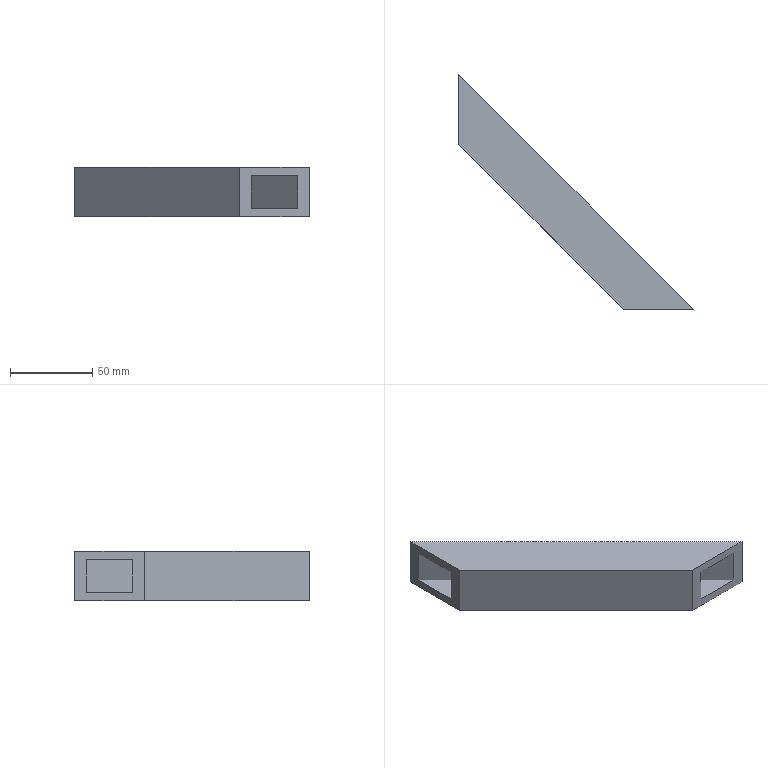Part | NX | features solid 2 | 1 solid | 10 faces | box 142.426 x 142.426 x 30 mm | volume 85711 mm3 | plane 10
STEP:
#1=CARTESIAN_POINT('',(347.426,-165.,-50.));
#2=VERTEX_POINT('',#1);
#3=CARTESIAN_POINT('',(347.426,-165.,-80.));
#4=VERTEX_POINT('',#3);
#5=CARTESIAN_POINT('',(347.426,-165.,-50.));
#6=DIRECTION('',(0.,0.,-1.));
#7=VECTOR('',#6,1000.);
#8=LINE('',#5,#7);
#9=EDGE_CURVE('',#2,#4,#8,.T.);
#10=ORIENTED_EDGE('',*,*,#9,.F.);
#11=CARTESIAN_POINT('',(305.,-165.,-50.));
#12=VERTEX_POINT('',#11);
#13=CARTESIAN_POINT('',(305.,-165.,-50.));
#14=DIRECTION('',(1.,0.,0.));
#15=VECTOR('',#14,1000.);
#16=LINE('',#13,#15);
#17=EDGE_CURVE('',#12,#2,#16,.T.);
#18=ORIENTED_EDGE('',*,*,#17,.F.);
#19=CARTESIAN_POINT('',(305.,-165.,-80.));
#20=VERTEX_POINT('',#19);
#21=CARTESIAN_POINT('',(305.,-165.,-50.));
#22=DIRECTION('',(0.,0.,1.));
#23=VECTOR('',#22,1000.);
#24=LINE('',#21,#23);
#25=EDGE_CURVE('',#12,#20,#24,.F.);
#26=ORIENTED_EDGE('',*,*,#25,.T.);
#27=CARTESIAN_POINT('',(140.,-165.,-80.));
#28=DIRECTION('',(-1.,0.,0.));
#29=VECTOR('',#28,1000.);
#30=LINE('',#27,#29);
#31=EDGE_CURVE('',#20,#4,#30,.F.);
#32=ORIENTED_EDGE('',*,*,#31,.T.);
#33=EDGE_LOOP('',(#10,#18,#26,#32));
#34=FACE_BOUND('',#33,.T.);
#35=CARTESIAN_POINT('',(340.355,-165.,-55.));
#36=VERTEX_POINT('',#35);
#37=CARTESIAN_POINT('',(340.355,-165.,-75.));
#38=VERTEX_POINT('',#37);
#39=CARTESIAN_POINT('',(340.355,-165.,-50.));
#40=DIRECTION('',(0.,0.,-1.));
#41=VECTOR('',#40,1000.);
#42=LINE('',#39,#41);
#43=EDGE_CURVE('',#36,#38,#42,.T.);
#44=ORIENTED_EDGE('',*,*,#43,.T.);
#45=CARTESIAN_POINT('',(312.071,-165.,-75.));
#46=VERTEX_POINT('',#45);
#47=CARTESIAN_POINT('',(140.,-165.,-75.));
#48=DIRECTION('',(-1.,0.,0.));
#49=VECTOR('',#48,1000.);
#50=LINE('',#47,#49);
#51=EDGE_CURVE('',#46,#38,#50,.F.);
#52=ORIENTED_EDGE('',*,*,#51,.F.);
#53=CARTESIAN_POINT('',(312.071,-165.,-55.));
#54=VERTEX_POINT('',#53);
#55=CARTESIAN_POINT('',(312.071,-165.,-50.));
#56=DIRECTION('',(0.,0.,1.));
#57=VECTOR('',#56,1000.);
#58=LINE('',#55,#57);
#59=EDGE_CURVE('',#54,#46,#58,.F.);
#60=ORIENTED_EDGE('',*,*,#59,.F.);
#61=CARTESIAN_POINT('',(305.,-165.,-55.));
#62=DIRECTION('',(1.,0.,0.));
#63=VECTOR('',#62,1000.);
#64=LINE('',#61,#63);
#65=EDGE_CURVE('',#54,#36,#64,.T.);
#66=ORIENTED_EDGE('',*,*,#65,.T.);
#67=EDGE_LOOP('',(#44,#52,#60,#66));
#68=FACE_BOUND('',#67,.T.);
#69=CARTESIAN_POINT('',(140.,-165.,-50.));
#70=DIRECTION('',(0.,-1.,0.));
#71=DIRECTION('',(0.,0.,-1.));
#72=AXIS2_PLACEMENT_3D('',#69,#70,#71);
#73=PLANE('',#72);
#74=ADVANCED_FACE('',(#34,#68),#73,.T.);
#75=CARTESIAN_POINT('',(205.,-22.574,-50.));
#76=VERTEX_POINT('',#75);
#77=CARTESIAN_POINT('',(205.,-22.574,-80.));
#78=VERTEX_POINT('',#77);
#79=CARTESIAN_POINT('',(205.,-22.574,-50.));
#80=DIRECTION('',(0.,0.,-1.));
#81=VECTOR('',#80,1000.);
#82=LINE('',#79,#81);
#83=EDGE_CURVE('',#76,#78,#82,.T.);
#84=ORIENTED_EDGE('',*,*,#83,.T.);
#85=CARTESIAN_POINT('',(205.,-65.,-80.));
#86=VERTEX_POINT('',#85);
#87=CARTESIAN_POINT('',(205.,20.,-80.));
#88=DIRECTION('',(0.,-1.,0.));
#89=VECTOR('',#88,1000.);
#90=LINE('',#87,#89);
#91=EDGE_CURVE('',#86,#78,#90,.F.);
#92=ORIENTED_EDGE('',*,*,#91,.F.);
#93=CARTESIAN_POINT('',(205.,-65.,-50.));
#94=VERTEX_POINT('',#93);
#95=CARTESIAN_POINT('',(205.,-65.,-50.));
#96=DIRECTION('',(0.,0.,1.));
#97=VECTOR('',#96,1000.);
#98=LINE('',#95,#97);
#99=EDGE_CURVE('',#94,#86,#98,.F.);
#100=ORIENTED_EDGE('',*,*,#99,.F.);
#101=CARTESIAN_POINT('',(205.,-165.,-50.));
#102=DIRECTION('',(0.,1.,0.));
#103=VECTOR('',#102,1000.);
#104=LINE('',#101,#103);
#105=EDGE_CURVE('',#94,#76,#104,.T.);
#106=ORIENTED_EDGE('',*,*,#105,.T.);
#107=EDGE_LOOP('',(#84,#92,#100,#106));
#108=FACE_BOUND('',#107,.T.);
#109=CARTESIAN_POINT('',(205.,-57.929,-55.));
#110=VERTEX_POINT('',#109);
#111=CARTESIAN_POINT('',(205.,-29.645,-55.));
#112=VERTEX_POINT('',#111);
#113=CARTESIAN_POINT('',(205.,-165.,-55.));
#114=DIRECTION('',(0.,1.,0.));
#115=VECTOR('',#114,1000.);
#116=LINE('',#113,#115);
#117=EDGE_CURVE('',#110,#112,#116,.T.);
#118=ORIENTED_EDGE('',*,*,#117,.F.);
#119=CARTESIAN_POINT('',(205.,-57.929,-75.));
#120=VERTEX_POINT('',#119);
#121=CARTESIAN_POINT('',(205.,-57.929,-50.));
#122=DIRECTION('',(0.,0.,1.));
#123=VECTOR('',#122,1000.);
#124=LINE('',#121,#123);
#125=EDGE_CURVE('',#110,#120,#124,.F.);
#126=ORIENTED_EDGE('',*,*,#125,.T.);
#127=CARTESIAN_POINT('',(205.,-29.645,-75.));
#128=VERTEX_POINT('',#127);
#129=CARTESIAN_POINT('',(205.,20.,-75.));
#130=DIRECTION('',(0.,-1.,0.));
#131=VECTOR('',#130,1000.);
#132=LINE('',#129,#131);
#133=EDGE_CURVE('',#120,#128,#132,.F.);
#134=ORIENTED_EDGE('',*,*,#133,.T.);
#135=CARTESIAN_POINT('',(205.,-29.645,-50.));
#136=DIRECTION('',(0.,0.,-1.));
#137=VECTOR('',#136,1000.);
#138=LINE('',#135,#137);
#139=EDGE_CURVE('',#112,#128,#138,.T.);
#140=ORIENTED_EDGE('',*,*,#139,.F.);
#141=EDGE_LOOP('',(#118,#126,#134,#140));
#142=FACE_BOUND('',#141,.T.);
#143=CARTESIAN_POINT('',(205.,20.,-50.));
#144=DIRECTION('',(1.,0.,0.));
#145=DIRECTION('',(0.,0.,1.));
#146=AXIS2_PLACEMENT_3D('',#143,#144,#145);
#147=PLANE('',#146);
#148=ADVANCED_FACE('',(#108,#142),#147,.F.);
#149=CARTESIAN_POINT('',(305.,-165.,-80.));
#150=DIRECTION('',(0.7071,-0.7071,0.));
#151=VECTOR('',#150,1000.);
#152=LINE('',#149,#151);
#153=EDGE_CURVE('',#86,#20,#152,.T.);
#154=ORIENTED_EDGE('',*,*,#153,.T.);
#155=ORIENTED_EDGE('',*,*,#25,.F.);
#156=CARTESIAN_POINT('',(305.,-165.,-50.));
#157=DIRECTION('',(0.7071,-0.7071,0.));
#158=VECTOR('',#157,1000.);
#159=LINE('',#156,#158);
#160=EDGE_CURVE('',#94,#12,#159,.T.);
#161=ORIENTED_EDGE('',*,*,#160,.F.);
#162=ORIENTED_EDGE('',*,*,#99,.T.);
#163=EDGE_LOOP('',(#154,#155,#161,#162));
#164=FACE_BOUND('',#163,.T.);
#165=CARTESIAN_POINT('',(305.,-165.,-50.));
#166=DIRECTION('',(-0.7071,-0.7071,0.));
#167=DIRECTION('',(0.,0.,-1.));
#168=AXIS2_PLACEMENT_3D('',#165,#166,#167);
#169=PLANE('',#168);
#170=ADVANCED_FACE('',(#164),#169,.T.);
#171=ORIENTED_EDGE('',*,*,#160,.T.);
#172=ORIENTED_EDGE('',*,*,#17,.T.);
#173=CARTESIAN_POINT('',(326.213,-143.787,-50.));
#174=DIRECTION('',(0.7071,-0.7071,0.));
#175=VECTOR('',#174,1000.);
#176=LINE('',#173,#175);
#177=EDGE_CURVE('',#76,#2,#176,.T.);
#178=ORIENTED_EDGE('',*,*,#177,.F.);
#179=ORIENTED_EDGE('',*,*,#105,.F.);
#180=EDGE_LOOP('',(#171,#172,#178,#179));
#181=FACE_BOUND('',#180,.T.);
#182=CARTESIAN_POINT('',(305.,-165.,-50.));
#183=DIRECTION('',(0.,0.,-1.));
#184=DIRECTION('',(0.7071,0.7071,0.));
#185=AXIS2_PLACEMENT_3D('',#182,#183,#184);
#186=PLANE('',#185);
#187=ADVANCED_FACE('',(#181),#186,.F.);
#188=ORIENTED_EDGE('',*,*,#177,.T.);
#189=ORIENTED_EDGE('',*,*,#9,.T.);
#190=CARTESIAN_POINT('',(326.213,-143.787,-80.));
#191=DIRECTION('',(0.7071,-0.7071,0.));
#192=VECTOR('',#191,1000.);
#193=LINE('',#190,#192);
#194=EDGE_CURVE('',#78,#4,#193,.T.);
#195=ORIENTED_EDGE('',*,*,#194,.F.);
#196=ORIENTED_EDGE('',*,*,#83,.F.);
#197=EDGE_LOOP('',(#188,#189,#195,#196));
#198=FACE_BOUND('',#197,.T.);
#199=CARTESIAN_POINT('',(326.213,-143.787,-50.));
#200=DIRECTION('',(-0.7071,-0.7071,0.));
#201=DIRECTION('',(0.,0.,-1.));
#202=AXIS2_PLACEMENT_3D('',#199,#200,#201);
#203=PLANE('',#202);
#204=ADVANCED_FACE('',(#198),#203,.F.);
#205=ORIENTED_EDGE('',*,*,#91,.T.);
#206=ORIENTED_EDGE('',*,*,#194,.T.);
#207=ORIENTED_EDGE('',*,*,#31,.F.);
#208=ORIENTED_EDGE('',*,*,#153,.F.);
#209=EDGE_LOOP('',(#205,#206,#207,#208));
#210=FACE_BOUND('',#209,.T.);
#211=CARTESIAN_POINT('',(305.,-165.,-80.));
#212=DIRECTION('',(0.,0.,-1.));
#213=DIRECTION('',(0.7071,0.7071,0.));
#214=AXIS2_PLACEMENT_3D('',#211,#212,#213);
#215=PLANE('',#214);
#216=ADVANCED_FACE('',(#210),#215,.T.);
#217=CARTESIAN_POINT('',(308.536,-161.464,-75.));
#218=DIRECTION('',(0.7071,-0.7071,0.));
#219=VECTOR('',#218,1000.);
#220=LINE('',#217,#219);
#221=EDGE_CURVE('',#120,#46,#220,.T.);
#222=ORIENTED_EDGE('',*,*,#221,.F.);
#223=ORIENTED_EDGE('',*,*,#125,.F.);
#224=CARTESIAN_POINT('',(308.536,-161.464,-55.));
#225=DIRECTION('',(-0.7071,0.7071,0.));
#226=VECTOR('',#225,1000.);
#227=LINE('',#224,#226);
#228=EDGE_CURVE('',#110,#54,#227,.F.);
#229=ORIENTED_EDGE('',*,*,#228,.T.);
#230=ORIENTED_EDGE('',*,*,#59,.T.);
#231=EDGE_LOOP('',(#222,#223,#229,#230));
#232=FACE_BOUND('',#231,.T.);
#233=CARTESIAN_POINT('',(308.536,-161.464,-50.));
#234=DIRECTION('',(-0.7071,-0.7071,0.));
#235=DIRECTION('',(0.,0.,-1.));
#236=AXIS2_PLACEMENT_3D('',#233,#234,#235);
#237=PLANE('',#236);
#238=ADVANCED_FACE('',(#232),#237,.F.);
#239=ORIENTED_EDGE('',*,*,#228,.F.);
#240=ORIENTED_EDGE('',*,*,#117,.T.);
#241=CARTESIAN_POINT('',(322.678,-147.322,-55.));
#242=DIRECTION('',(0.7071,-0.7071,0.));
#243=VECTOR('',#242,1000.);
#244=LINE('',#241,#243);
#245=EDGE_CURVE('',#112,#36,#244,.T.);
#246=ORIENTED_EDGE('',*,*,#245,.T.);
#247=ORIENTED_EDGE('',*,*,#65,.F.);
#248=EDGE_LOOP('',(#239,#240,#246,#247));
#249=FACE_BOUND('',#248,.T.);
#250=CARTESIAN_POINT('',(305.,-165.,-55.));
#251=DIRECTION('',(0.,0.,-1.));
#252=DIRECTION('',(0.7071,0.7071,0.));
#253=AXIS2_PLACEMENT_3D('',#250,#251,#252);
#254=PLANE('',#253);
#255=ADVANCED_FACE('',(#249),#254,.T.);
#256=ORIENTED_EDGE('',*,*,#245,.F.);
#257=ORIENTED_EDGE('',*,*,#139,.T.);
#258=CARTESIAN_POINT('',(322.678,-147.322,-75.));
#259=DIRECTION('',(-0.7071,0.7071,0.));
#260=VECTOR('',#259,1000.);
#261=LINE('',#258,#260);
#262=EDGE_CURVE('',#128,#38,#261,.F.);
#263=ORIENTED_EDGE('',*,*,#262,.T.);
#264=ORIENTED_EDGE('',*,*,#43,.F.);
#265=EDGE_LOOP('',(#256,#257,#263,#264));
#266=FACE_BOUND('',#265,.T.);
#267=CARTESIAN_POINT('',(322.678,-147.322,-50.));
#268=DIRECTION('',(-0.7071,-0.7071,0.));
#269=DIRECTION('',(0.,0.,-1.));
#270=AXIS2_PLACEMENT_3D('',#267,#268,#269);
#271=PLANE('',#270);
#272=ADVANCED_FACE('',(#266),#271,.T.);
#273=ORIENTED_EDGE('',*,*,#133,.F.);
#274=ORIENTED_EDGE('',*,*,#221,.T.);
#275=ORIENTED_EDGE('',*,*,#51,.T.);
#276=ORIENTED_EDGE('',*,*,#262,.F.);
#277=EDGE_LOOP('',(#273,#274,#275,#276));
#278=FACE_BOUND('',#277,.T.);
#279=CARTESIAN_POINT('',(305.,-165.,-75.));
#280=DIRECTION('',(0.,0.,-1.));
#281=DIRECTION('',(0.7071,0.7071,0.));
#282=AXIS2_PLACEMENT_3D('',#279,#280,#281);
#283=PLANE('',#282);
#284=ADVANCED_FACE('',(#278),#283,.F.);
#285=CLOSED_SHELL('',(#74,#148,#170,#187,#204,#216,#238,#255,#272,#284));
#286=MANIFOLD_SOLID_BREP('',#285);
#287=(LENGTH_UNIT()NAMED_UNIT(*)SI_UNIT(.MILLI.,.METRE.));
#288=UNCERTAINTY_MEASURE_WITH_UNIT(LENGTH_MEASURE(0.00001),#287,'','');
#289=(NAMED_UNIT(*)PLANE_ANGLE_UNIT()SI_UNIT($,.RADIAN.));
#290=(NAMED_UNIT(*)SI_UNIT($,.STERADIAN.)SOLID_ANGLE_UNIT());
#291=(GEOMETRIC_REPRESENTATION_CONTEXT(3)GLOBAL_UNCERTAINTY_ASSIGNED_CONTEXT((#288))GLOBAL_UNIT_ASSIGNED_CONTEXT((#287,#289,#290))REPRESENTATION_CONTEXT('',''));
#292=ADVANCED_BREP_SHAPE_REPRESENTATION('',(#286),#291);